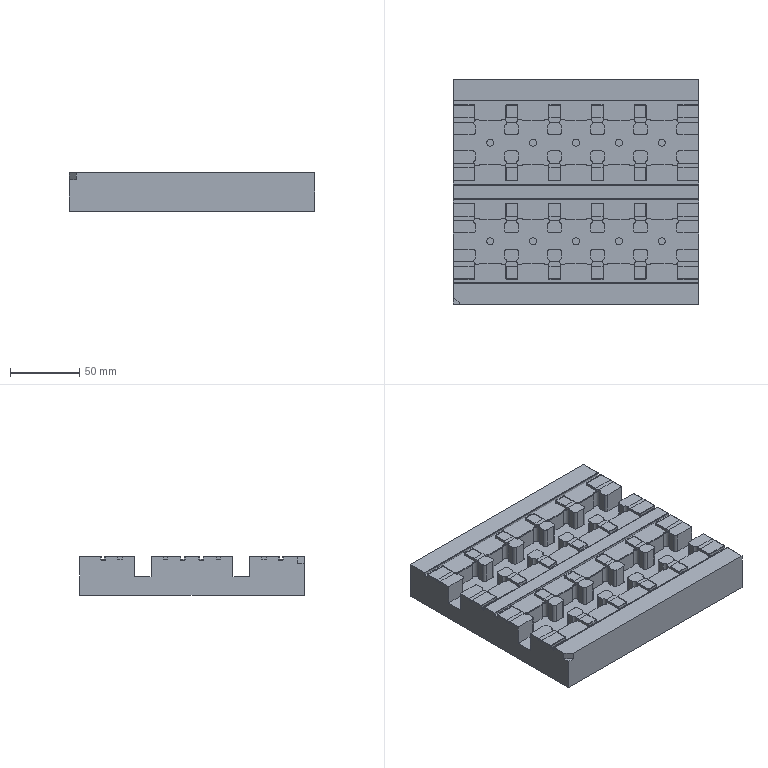NC program | NX | posted by the shop | part box 177 x 162 x 28 mm
Lines 685 to 1998 of 240480:
N4 T10 M06
(D10  D=10. R=0. H=10 ce=0.15 di=0.06)
(MAX_Z=43. MIN_Z=13.56 Time=54.07M)
T05
G00 G90 G54 X96.5 Y35.6 M03 S3000
G43 H10 Z43.
M08
Z28.551
G01 Z28.051 F2000.
X89.5
Y34.75
X74.25
G03 X67.1 Y27.6 I0.0 J-7.15
G01 Y24.98
X56.9
Y27.6
G03 X49.75 Y34.75 I-7.15 J0.0
G01 X43.25
G03 X36.1 Y27.6 I0.0 J-7.15
G01 Y24.98
X25.9
Y27.6
G03 X18.75 Y34.75 I-7.15 J0.0
G01 X12.25
G03 X5.1 Y27.6 I0.0 J-7.15
G01 Y24.98
X-5.1
Y27.6
G03 X-12.25 Y34.75 I-7.15 J0.0
G01 X-18.75
G03 X-25.9 Y27.6 I0.0 J-7.15
G01 Y24.98
X-36.1
Y27.6
G03 X-43.25 Y34.75 I-7.15 J0.0
G01 X-49.75
G03 X-56.9 Y27.6 I0.0 J-7.15
G01 Y24.98
X-67.1
Y27.6
G03 X-74.25 Y34.75 I-7.15 J0.0
G01 X-89.5
Y36.45
X-74.25
G03 X-67.1 Y43.6 I0.0 J7.15
G01 Y46.22
X-56.9
Y43.6
G03 X-55.648 Y39.558 I7.15 J0.0
G01 X-61.421 Y35.6
G03 X-62. Y34.682 I11.671 J-8.
X-62.579 Y35.6 I-12.25 J-7.082
X-62. Y36.518 I-11.671 J8.
X-61.421 Y35.6 I12.25 J7.082
G01 X-55.648 Y39.558
G03 X-49.75 Y36.45 I5.898 J4.042
G01 X-43.25
G03 X-36.1 Y43.6 I0.0 J7.15
G01 Y46.22
X-25.9
Y43.6
G03 X-24.648 Y39.558 I7.15 J0.0
G01 X-30.421 Y35.6
G03 X-31. Y34.682 I11.671 J-8.
X-31.579 Y35.6 I-12.25 J-7.082
X-31. Y36.518 I-11.671 J8.
X-30.421 Y35.6 I12.25 J7.082
G01 X-24.648 Y39.558
G03 X-18.75 Y36.45 I5.898 J4.042
G01 X-12.25
G03 X-5.1 Y43.6 I0.0 J7.15
G01 Y46.22
X5.1
Y43.6
G03 X6.352 Y39.558 I7.15 J0.0
G01 X.579 Y35.6
G03 X0.0 Y34.682 I11.671 J-8.
X-.579 Y35.6 I-12.25 J-7.082
X0.0 Y36.518 I-11.671 J8.
X.579 Y35.6 I12.25 J7.082
G01 X6.352 Y39.558
G03 X12.25 Y36.45 I5.898 J4.042
G01 X18.75
G03 X25.9 Y43.6 I0.0 J7.15
G01 Y46.22
X36.1
Y43.6
G03 X37.352 Y39.558 I7.15 J0.0
G01 X31.579 Y35.6
G03 X31. Y34.682 I11.671 J-8.
X30.421 Y35.6 I-12.25 J-7.082
X31. Y36.518 I-11.671 J8.
X31.579 Y35.6 I12.25 J7.082
G01 X37.352 Y39.558
G03 X43.25 Y36.45 I5.898 J4.042
G01 X49.75
G03 X56.9 Y43.6 I0.0 J7.15
G01 Y46.22
X67.1
Y43.6
G03 X68.352 Y39.558 I7.15 J0.0
G01 X62.579 Y35.6
G03 X62. Y34.682 I11.671 J-8.
X61.421 Y35.6 I-12.25 J-7.082
X62. Y36.518 I-11.671 J8.
X62.579 Y35.6 I12.25 J7.082
G01 X68.352 Y39.558
G03 X74.25 Y36.45 I5.898 J4.042
G01 X89.5
Y35.6
Y35.1
Z28.551
G00 Z43.
X96.65 Y35.6
Z28.353
G01 Z27.853
X89.5
Y34.75
X74.25
G03 X67.1 Y27.6 I0.0 J-7.15
G01 Y24.98
X56.9
Y27.6
G03 X49.75 Y34.75 I-7.15 J0.0
G01 X43.25
G03 X36.1 Y27.6 I0.0 J-7.15
G01 Y24.98
X25.9
Y27.6
G03 X18.75 Y34.75 I-7.15 J0.0
G01 X12.25
G03 X5.1 Y27.6 I0.0 J-7.15
G01 Y24.98
X-5.1
Y27.6
G03 X-12.25 Y34.75 I-7.15 J0.0
G01 X-18.75
G03 X-25.9 Y27.6 I0.0 J-7.15
G01 Y24.98
X-36.1
Y27.6
G03 X-43.25 Y34.75 I-7.15 J0.0
G01 X-49.75
G03 X-56.9 Y27.6 I0.0 J-7.15
G01 Y24.98
X-67.1
Y27.6
G03 X-74.25 Y34.75 I-7.15 J0.0
G01 X-89.5
Y36.45
X-74.25
G03 X-67.1 Y43.6 I0.0 J7.15
G01 Y46.22
X-56.9
Y43.6
G03 X-55.648 Y39.558 I7.15 J0.0
G01 X-61.421 Y35.6
G03 X-62. Y34.682 I11.671 J-8.
X-62.579 Y35.6 I-12.25 J-7.082
X-62. Y36.518 I-11.671 J8.
X-61.421 Y35.6 I12.25 J7.082
G01 X-55.648 Y39.558
G03 X-49.75 Y36.45 I5.898 J4.042
G01 X-43.25
G03 X-36.1 Y43.6 I0.0 J7.15
G01 Y46.22
X-25.9
Y43.6
G03 X-24.648 Y39.558 I7.15 J0.0
G01 X-30.421 Y35.6
G03 X-31. Y34.682 I11.671 J-8.
X-31.579 Y35.6 I-12.25 J-7.082
X-31. Y36.518 I-11.671 J8.
X-30.421 Y35.6 I12.25 J7.082
G01 X-24.648 Y39.558
G03 X-18.75 Y36.45 I5.898 J4.042
G01 X-12.25
G03 X-5.1 Y43.6 I0.0 J7.15
G01 Y46.22
X5.1
Y43.6
G03 X6.352 Y39.558 I7.15 J0.0
G01 X.579 Y35.6
G03 X0.0 Y34.682 I11.671 J-8.
X-.579 Y35.6 I-12.25 J-7.082
X0.0 Y36.518 I-11.671 J8.
X.579 Y35.6 I12.25 J7.082
G01 X6.352 Y39.558
G03 X12.25 Y36.45 I5.898 J4.042
G01 X18.75
G03 X25.9 Y43.6 I0.0 J7.15
G01 Y46.22
X36.1
Y43.6
G03 X37.352 Y39.558 I7.15 J0.0
G01 X31.579 Y35.6
G03 X31. Y34.682 I11.671 J-8.
X30.421 Y35.6 I-12.25 J-7.082
X31. Y36.518 I-11.671 J8.
X31.579 Y35.6 I12.25 J7.082
G01 X37.352 Y39.558
G03 X43.25 Y36.45 I5.898 J4.042
G01 X49.75
G03 X56.9 Y43.6 I0.0 J7.15
G01 Y46.22
X67.1
Y43.6
G03 X68.352 Y39.558 I7.15 J0.0
G01 X62.579 Y35.6
G03 X62. Y34.682 I11.671 J-8.
X61.421 Y35.6 I-12.25 J-7.082
X62. Y36.518 I-11.671 J8.
X62.579 Y35.6 I12.25 J7.082
G01 X68.352 Y39.558
G03 X74.25 Y36.45 I5.898 J4.042
G01 X89.5
Y35.6
Y35.1
Z28.353
G00 Z28.551
X96.65 Y35.6
Z28.154
G01 Z27.654
X89.5
Y34.75
X74.25
G03 X67.1 Y27.6 I0.0 J-7.15
G01 Y24.98
X56.9
Y27.6
G03 X49.75 Y34.75 I-7.15 J0.0
G01 X43.25
G03 X36.1 Y27.6 I0.0 J-7.15
G01 Y24.98
X25.9
Y27.6
G03 X18.75 Y34.75 I-7.15 J0.0
G01 X12.25
G03 X5.1 Y27.6 I0.0 J-7.15
G01 Y24.98
X-5.1
Y27.6
G03 X-12.25 Y34.75 I-7.15 J0.0
G01 X-18.75
G03 X-25.9 Y27.6 I0.0 J-7.15
G01 Y24.98
X-36.1
Y27.6
G03 X-43.25 Y34.75 I-7.15 J0.0
G01 X-49.75
G03 X-56.9 Y27.6 I0.0 J-7.15
G01 Y24.98
X-67.1
Y27.6
G03 X-74.25 Y34.75 I-7.15 J0.0
G01 X-89.5
Y36.45
X-74.25
G03 X-67.1 Y43.6 I0.0 J7.15
G01 Y46.22
X-56.9
Y43.6
G03 X-55.648 Y39.558 I7.15 J0.0
G01 X-61.421 Y35.6
G03 X-62. Y34.682 I11.671 J-8.
X-62.579 Y35.6 I-12.25 J-7.082
X-62. Y36.518 I-11.671 J8.
X-61.421 Y35.6 I12.25 J7.082
G01 X-55.648 Y39.558
G03 X-49.75 Y36.45 I5.898 J4.042
G01 X-43.25
G03 X-36.1 Y43.6 I0.0 J7.15
G01 Y46.22
X-25.9
Y43.6
G03 X-24.648 Y39.558 I7.15 J0.0
G01 X-30.421 Y35.6
G03 X-31. Y34.682 I11.671 J-8.
X-31.579 Y35.6 I-12.25 J-7.082
X-31. Y36.518 I-11.671 J8.
X-30.421 Y35.6 I12.25 J7.082
G01 X-24.648 Y39.558
G03 X-18.75 Y36.45 I5.898 J4.042
G01 X-12.25
G03 X-5.1 Y43.6 I0.0 J7.15
G01 Y46.22
X5.1
Y43.6
G03 X6.352 Y39.558 I7.15 J0.0
G01 X.579 Y35.6
G03 X0.0 Y34.682 I11.671 J-8.
X-.579 Y35.6 I-12.25 J-7.082
X0.0 Y36.518 I-11.671 J8.
X.579 Y35.6 I12.25 J7.082
G01 X6.352 Y39.558
G03 X12.25 Y36.45 I5.898 J4.042
G01 X18.75
G03 X25.9 Y43.6 I0.0 J7.15
G01 Y46.22
X36.1
Y43.6
G03 X37.352 Y39.558 I7.15 J0.0
G01 X31.579 Y35.6
G03 X31. Y34.682 I11.671 J-8.
X30.421 Y35.6 I-12.25 J-7.082
X31. Y36.518 I-11.671 J8.
X31.579 Y35.6 I12.25 J7.082
G01 X37.352 Y39.558
G03 X43.25 Y36.45 I5.898 J4.042
G01 X49.75
G03 X56.9 Y43.6 I0.0 J7.15
G01 Y46.22
X67.1
Y43.6
G03 X68.352 Y39.558 I7.15 J0.0
G01 X62.579 Y35.6
G03 X62. Y34.682 I11.671 J-8.
X61.421 Y35.6 I-12.25 J-7.082
X62. Y36.518 I-11.671 J8.
X62.579 Y35.6 I12.25 J7.082
G01 X68.352 Y39.558
G03 X74.25 Y36.45 I5.898 J4.042
G01 X89.5
Y35.6
Y35.1
Z28.154
G00 Z28.353
X96.65 Y35.6
Z27.956
G01 Z27.456
X89.5
Y34.75
X74.25
G03 X67.1 Y27.6 I0.0 J-7.15
G01 Y24.98
X56.9
Y27.6
G03 X49.75 Y34.75 I-7.15 J0.0
G01 X43.25
G03 X36.1 Y27.6 I0.0 J-7.15
G01 Y24.98
X25.9
Y27.6
G03 X18.75 Y34.75 I-7.15 J0.0
G01 X12.25
G03 X5.1 Y27.6 I0.0 J-7.15
G01 Y24.98
X-5.1
Y27.6
G03 X-12.25 Y34.75 I-7.15 J0.0
G01 X-18.75
G03 X-25.9 Y27.6 I0.0 J-7.15
G01 Y24.98
X-36.1
Y27.6
G03 X-43.25 Y34.75 I-7.15 J0.0
G01 X-49.75
G03 X-56.9 Y27.6 I0.0 J-7.15
G01 Y24.98
X-67.1
Y27.6
G03 X-74.25 Y34.75 I-7.15 J0.0
G01 X-89.5
Y36.45
X-74.25
G03 X-67.1 Y43.6 I0.0 J7.15
G01 Y46.22
X-56.9
Y43.6
G03 X-55.648 Y39.558 I7.15 J0.0
G01 X-61.421 Y35.6
G03 X-62. Y34.682 I11.671 J-8.
X-62.579 Y35.6 I-12.25 J-7.082
X-62. Y36.518 I-11.671 J8.
X-61.421 Y35.6 I12.25 J7.082
G01 X-55.648 Y39.558
G03 X-49.75 Y36.45 I5.898 J4.042
G01 X-43.25
G03 X-36.1 Y43.6 I0.0 J7.15
G01 Y46.22
X-25.9
Y43.6
G03 X-24.648 Y39.558 I7.15 J0.0
G01 X-30.421 Y35.6
G03 X-31. Y34.682 I11.671 J-8.
X-31.579 Y35.6 I-12.25 J-7.082
X-31. Y36.518 I-11.671 J8.
X-30.421 Y35.6 I12.25 J7.082
G01 X-24.648 Y39.558
G03 X-18.75 Y36.45 I5.898 J4.042
G01 X-12.25
G03 X-5.1 Y43.6 I0.0 J7.15
G01 Y46.22
X5.1
Y43.6
G03 X6.352 Y39.558 I7.15 J0.0
G01 X.579 Y35.6
G03 X0.0 Y34.682 I11.671 J-8.
X-.579 Y35.6 I-12.25 J-7.082
X0.0 Y36.518 I-11.671 J8.
X.579 Y35.6 I12.25 J7.082
G01 X6.352 Y39.558
G03 X12.25 Y36.45 I5.898 J4.042
G01 X18.75
G03 X25.9 Y43.6 I0.0 J7.15
G01 Y46.22
X36.1
Y43.6
G03 X37.352 Y39.558 I7.15 J0.0
G01 X31.579 Y35.6
G03 X31. Y34.682 I11.671 J-8.
X30.421 Y35.6 I-12.25 J-7.082
X31. Y36.518 I-11.671 J8.
X31.579 Y35.6 I12.25 J7.082
G01 X37.352 Y39.558
G03 X43.25 Y36.45 I5.898 J4.042
G01 X49.75
G03 X56.9 Y43.6 I0.0 J7.15
G01 Y46.22
X67.1
Y43.6
G03 X68.352 Y39.558 I7.15 J0.0
G01 X62.579 Y35.6
G03 X62. Y34.682 I11.671 J-8.
X61.421 Y35.6 I-12.25 J-7.082
X62. Y36.518 I-11.671 J8.
X62.579 Y35.6 I12.25 J7.082
G01 X68.352 Y39.558
G03 X74.25 Y36.45 I5.898 J4.042
G01 X89.5
Y35.6
Y35.1
Z27.956
G00 Z28.154
X96.65 Y35.6
Z27.757
G01 Z27.257
X89.5
Y34.75
X74.25
G03 X67.1 Y27.6 I0.0 J-7.15
G01 Y24.98
X56.9
Y27.6
G03 X49.75 Y34.75 I-7.15 J0.0
G01 X43.25
G03 X36.1 Y27.6 I0.0 J-7.15
G01 Y24.98
X25.9
Y27.6
G03 X18.75 Y34.75 I-7.15 J0.0
G01 X12.25
G03 X5.1 Y27.6 I0.0 J-7.15
G01 Y24.98
X-5.1
Y27.6
G03 X-12.25 Y34.75 I-7.15 J0.0
G01 X-18.75
G03 X-25.9 Y27.6 I0.0 J-7.15
G01 Y24.98
X-36.1
Y27.6
G03 X-43.25 Y34.75 I-7.15 J0.0
G01 X-49.75
G03 X-56.9 Y27.6 I0.0 J-7.15
G01 Y24.98
X-67.1
Y27.6
G03 X-74.25 Y34.75 I-7.15 J0.0
G01 X-89.5
Y36.45
X-74.25
G03 X-67.1 Y43.6 I0.0 J7.15
G01 Y46.22
X-56.9
Y43.6
G03 X-55.648 Y39.558 I7.15 J0.0
G01 X-61.421 Y35.6
G03 X-62. Y34.682 I11.671 J-8.
X-62.579 Y35.6 I-12.25 J-7.082
X-62. Y36.518 I-11.671 J8.
X-61.421 Y35.6 I12.25 J7.082
G01 X-55.648 Y39.558
G03 X-49.75 Y36.45 I5.898 J4.042
G01 X-43.25
G03 X-36.1 Y43.6 I0.0 J7.15
G01 Y46.22
X-25.9
Y43.6
G03 X-24.648 Y39.558 I7.15 J0.0
G01 X-30.421 Y35.6
G03 X-31. Y34.682 I11.671 J-8.
X-31.579 Y35.6 I-12.25 J-7.082
X-31. Y36.518 I-11.671 J8.
X-30.421 Y35.6 I12.25 J7.082
G01 X-24.648 Y39.558
G03 X-18.75 Y36.45 I5.898 J4.042
G01 X-12.25
G03 X-5.1 Y43.6 I0.0 J7.15
G01 Y46.22
X5.1
Y43.6
G03 X6.352 Y39.558 I7.15 J0.0
G01 X.579 Y35.6
G03 X0.0 Y34.682 I11.671 J-8.
X-.579 Y35.6 I-12.25 J-7.082
X0.0 Y36.518 I-11.671 J8.
X.579 Y35.6 I12.25 J7.082
G01 X6.352 Y39.558
G03 X12.25 Y36.45 I5.898 J4.042
G01 X18.75
G03 X25.9 Y43.6 I0.0 J7.15
G01 Y46.22
X36.1
Y43.6
G03 X37.352 Y39.558 I7.15 J0.0
G01 X31.579 Y35.6
G03 X31. Y34.682 I11.671 J-8.
X30.421 Y35.6 I-12.25 J-7.082
X31. Y36.518 I-11.671 J8.
X31.579 Y35.6 I12.25 J7.082
G01 X37.352 Y39.558
G03 X43.25 Y36.45 I5.898 J4.042
G01 X49.75
G03 X56.9 Y43.6 I0.0 J7.15
G01 Y46.22
X67.1
Y43.6
G03 X68.352 Y39.558 I7.15 J0.0
G01 X62.579 Y35.6
G03 X62. Y34.682 I11.671 J-8.
X61.421 Y35.6 I-12.25 J-7.082
X62. Y36.518 I-11.671 J8.
X62.579 Y35.6 I12.25 J7.082
G01 X68.352 Y39.558
G03 X74.25 Y36.45 I5.898 J4.042
G01 X89.5
Y35.6
Y35.1
Z27.757
G00 Z27.956
X96.65 Y35.6
Z27.559
G01 Z27.059
X89.5
Y34.75
X74.25
G03 X67.1 Y27.6 I0.0 J-7.15
G01 Y24.98
X56.9
Y27.6
G03 X49.75 Y34.75 I-7.15 J0.0
G01 X43.25
G03 X36.1 Y27.6 I0.0 J-7.15
G01 Y24.98
X25.9
Y27.6
G03 X18.75 Y34.75 I-7.15 J0.0
G01 X12.25
G03 X5.1 Y27.6 I0.0 J-7.15
G01 Y24.98
X-5.1
Y27.6
G03 X-12.25 Y34.75 I-7.15 J0.0
G01 X-18.75
G03 X-25.9 Y27.6 I0.0 J-7.15
G01 Y24.98
X-36.1
Y27.6
G03 X-43.25 Y34.75 I-7.15 J0.0
G01 X-49.75
G03 X-56.9 Y27.6 I0.0 J-7.15
G01 Y24.98
X-67.1
Y27.6
G03 X-74.25 Y34.75 I-7.15 J0.0
G01 X-89.5
Y36.45
X-74.25
G03 X-67.1 Y43.6 I0.0 J7.15
G01 Y46.22
X-56.9
Y43.6
G03 X-55.648 Y39.558 I7.15 J0.0
G01 X-61.421 Y35.6
G03 X-62. Y34.682 I11.671 J-8.
X-62.579 Y35.6 I-12.25 J-7.082
X-62. Y36.518 I-11.671 J8.
X-61.421 Y35.6 I12.25 J7.082
G01 X-55.648 Y39.558
G03 X-49.75 Y36.45 I5.898 J4.042
G01 X-43.25
G03 X-36.1 Y43.6 I0.0 J7.15
G01 Y46.22
X-25.9
Y43.6
G03 X-24.648 Y39.558 I7.15 J0.0
G01 X-30.421 Y35.6
G03 X-31. Y34.682 I11.671 J-8.
X-31.579 Y35.6 I-12.25 J-7.082
X-31. Y36.518 I-11.671 J8.
X-30.421 Y35.6 I12.25 J7.082
G01 X-24.648 Y39.558
G03 X-18.75 Y36.45 I5.898 J4.042
G01 X-12.25
G03 X-5.1 Y43.6 I0.0 J7.15
G01 Y46.22
X5.1
Y43.6
G03 X6.352 Y39.558 I7.15 J0.0
G01 X.579 Y35.6
G03 X0.0 Y34.682 I11.671 J-8.
X-.579 Y35.6 I-12.25 J-7.082
X0.0 Y36.518 I-11.671 J8.
X.579 Y35.6 I12.25 J7.082
G01 X6.352 Y39.558
G03 X12.25 Y36.45 I5.898 J4.042
G01 X18.75
G03 X25.9 Y43.6 I0.0 J7.15
G01 Y46.22
X36.1
Y43.6
G03 X37.352 Y39.558 I7.15 J0.0
G01 X31.579 Y35.6
G03 X31. Y34.682 I11.671 J-8.
X30.421 Y35.6 I-12.25 J-7.082
X31. Y36.518 I-11.671 J8.
X31.579 Y35.6 I12.25 J7.082
G01 X37.352 Y39.558
G03 X43.25 Y36.45 I5.898 J4.042
G01 X49.75
G03 X56.9 Y43.6 I0.0 J7.15
G01 Y46.22
X67.1
Y43.6
G03 X68.352 Y39.558 I7.15 J0.0
G01 X62.579 Y35.6
G03 X62. Y34.682 I11.671 J-8.
X61.421 Y35.6 I-12.25 J-7.082
X62. Y36.518 I-11.671 J8.
X62.579 Y35.6 I12.25 J7.082
G01 X68.352 Y39.558
G03 X74.25 Y36.45 I5.898 J4.042
G01 X89.5
Y35.6
Y35.1
Z27.559
G00 Z27.757
X96.65 Y35.6
Z27.36
G01 Z26.86
X89.5
Y34.75
X74.25
G03 X67.1 Y27.6 I0.0 J-7.15
G01 Y24.98
X56.9
Y27.6
G03 X49.75 Y34.75 I-7.15 J0.0
G01 X43.25
G03 X36.1 Y27.6 I0.0 J-7.15
G01 Y24.98
X25.9
Y27.6
G03 X18.75 Y34.75 I-7.15 J0.0
G01 X12.25
G03 X5.1 Y27.6 I0.0 J-7.15
G01 Y24.98
X-5.1
Y27.6
G03 X-12.25 Y34.75 I-7.15 J0.0
G01 X-18.75
G03 X-25.9 Y27.6 I0.0 J-7.15
G01 Y24.98
X-36.1
Y27.6
G03 X-43.25 Y34.75 I-7.15 J0.0
G01 X-49.75
G03 X-56.9 Y27.6 I0.0 J-7.15
G01 Y24.98
X-67.1
Y27.6
G03 X-74.25 Y34.75 I-7.15 J0.0
G01 X-89.5
Y36.45
X-74.25
G03 X-67.1 Y43.6 I0.0 J7.15
G01 Y46.22
X-56.9
Y43.6
G03 X-55.648 Y39.558 I7.15 J0.0
G01 X-61.421 Y35.6
G03 X-62. Y34.682 I11.671 J-8.
X-62.579 Y35.6 I-12.25 J-7.082
X-62. Y36.518 I-11.671 J8.
X-61.421 Y35.6 I12.25 J7.082
G01 X-55.648 Y39.558
G03 X-49.75 Y36.45 I5.898 J4.042
G01 X-43.25
G03 X-36.1 Y43.6 I0.0 J7.15
G01 Y46.22
X-25.9
Y43.6
G03 X-24.648 Y39.558 I7.15 J0.0
G01 X-30.421 Y35.6
G03 X-31. Y34.682 I11.671 J-8.
X-31.579 Y35.6 I-12.25 J-7.082
X-31. Y36.518 I-11.671 J8.
X-30.421 Y35.6 I12.25 J7.082
G01 X-24.648 Y39.558
G03 X-18.75 Y36.45 I5.898 J4.042
G01 X-12.25
G03 X-5.1 Y43.6 I0.0 J7.15
G01 Y46.22
X5.1
Y43.6
G03 X6.352 Y39.558 I7.15 J0.0
G01 X.579 Y35.6
G03 X0.0 Y34.682 I11.671 J-8.
X-.579 Y35.6 I-12.25 J-7.082
X0.0 Y36.518 I-11.671 J8.
X.579 Y35.6 I12.25 J7.082
G01 X6.352 Y39.558
G03 X12.25 Y36.45 I5.898 J4.042
G01 X18.75
G03 X25.9 Y43.6 I0.0 J7.15
G01 Y46.22
X36.1
Y43.6
G03 X37.352 Y39.558 I7.15 J0.0
G01 X31.579 Y35.6
G03 X31. Y34.682 I11.671 J-8.
X30.421 Y35.6 I-12.25 J-7.082
X31. Y36.518 I-11.671 J8.
X31.579 Y35.6 I12.25 J7.082
G01 X37.352 Y39.558
G03 X43.25 Y36.45 I5.898 J4.042
G01 X49.75
G03 X56.9 Y43.6 I0.0 J7.15
G01 Y46.22
X67.1
Y43.6
G03 X68.352 Y39.558 I7.15 J0.0
G01 X62.579 Y35.6
G03 X62. Y34.682 I11.671 J-8.
X61.421 Y35.6 I-12.25 J-7.082
X62. Y36.518 I-11.671 J8.
X62.579 Y35.6 I12.25 J7.082
G01 X68.352 Y39.558
G03 X74.25 Y36.45 I5.898 J4.042
G01 X89.5
Y35.6
Y35.1
Z27.36
G00 Z27.559
X96.65 Y35.6
Z27.162
G01 Z26.662
X89.5
Y34.75
X74.25
G03 X67.1 Y27.6 I0.0 J-7.15
G01 Y24.98
X56.9
Y27.6
G03 X49.75 Y34.75 I-7.15 J0.0
G01 X43.25
G03 X36.1 Y27.6 I0.0 J-7.15
G01 Y24.98
X25.9
Y27.6
G03 X18.75 Y34.75 I-7.15 J0.0
G01 X12.25
G03 X5.1 Y27.6 I0.0 J-7.15
G01 Y24.98
X-5.1
Y27.6
G03 X-12.25 Y34.75 I-7.15 J0.0
G01 X-18.75
G03 X-25.9 Y27.6 I0.0 J-7.15
G01 Y24.98
X-36.1
Y27.6
G03 X-43.25 Y34.75 I-7.15 J0.0
G01 X-49.75
G03 X-56.9 Y27.6 I0.0 J-7.15
G01 Y24.98
X-67.1
Y27.6
G03 X-74.25 Y34.75 I-7.15 J0.0
G01 X-89.5
Y36.45
X-74.25
G03 X-67.1 Y43.6 I0.0 J7.15
G01 Y46.22
X-56.9
Y43.6
G03 X-55.648 Y39.558 I7.15 J0.0
G01 X-61.421 Y35.6
G03 X-62. Y34.682 I11.671 J-8.
X-62.579 Y35.6 I-12.25 J-7.082
X-62. Y36.518 I-11.671 J8.
X-61.421 Y35.6 I12.25 J7.082
G01 X-55.648 Y39.558
G03 X-49.75 Y36.45 I5.898 J4.042
G01 X-43.25
G03 X-36.1 Y43.6 I0.0 J7.15
G01 Y46.22
X-25.9
Y43.6
G03 X-24.648 Y39.558 I7.15 J0.0
G01 X-30.421 Y35.6
G03 X-31. Y34.682 I11.671 J-8.
X-31.579 Y35.6 I-12.25 J-7.082
X-31. Y36.518 I-11.671 J8.
X-30.421 Y35.6 I12.25 J7.082
G01 X-24.648 Y39.558
G03 X-18.75 Y36.45 I5.898 J4.042
G01 X-12.25
G03 X-5.1 Y43.6 I0.0 J7.15
G01 Y46.22
X5.1
Y43.6
G03 X6.352 Y39.558 I7.15 J0.0
G01 X.579 Y35.6
G03 X0.0 Y34.682 I11.671 J-8.
X-.579 Y35.6 I-12.25 J-7.082
X0.0 Y36.518 I-11.671 J8.
X.579 Y35.6 I12.25 J7.082
G01 X6.352 Y39.558
G03 X12.25 Y36.45 I5.898 J4.042
G01 X18.75
G03 X25.9 Y43.6 I0.0 J7.15
G01 Y46.22
X36.1
Y43.6
G03 X37.352 Y39.558 I7.15 J0.0
G01 X31.579 Y35.6
G03 X31. Y34.682 I11.671 J-8.
X30.421 Y35.6 I-12.25 J-7.082
X31. Y36.518 I-11.671 J8.
X31.579 Y35.6 I12.25 J7.082
G01 X37.352 Y39.558
G03 X43.25 Y36.45 I5.898 J4.042
G01 X49.75
G03 X56.9 Y43.6 I0.0 J7.15
G01 Y46.22
X67.1
Y43.6
G03 X68.352 Y39.558 I7.15 J0.0
G01 X62.579 Y35.6
G03 X62. Y34.682 I11.671 J-8.
X61.421 Y35.6 I-12.25 J-7.082
X62. Y36.518 I-11.671 J8.
X62.579 Y35.6 I12.25 J7.082
G01 X68.352 Y39.558
G03 X74.25 Y36.45 I5.898 J4.042
G01 X89.5
Y35.6
Y35.1
Z27.162
G00 Z27.36
X96.65 Y35.6
Z26.963
G01 Z26.463
X89.5
Y34.75
X74.25
G03 X67.1 Y27.6 I0.0 J-7.15
G01 Y24.98
X56.9
Y27.6
G03 X49.75 Y34.75 I-7.15 J0.0
G01 X43.25
G03 X36.1 Y27.6 I0.0 J-7.15
G01 Y24.98
X25.9
Y27.6
G03 X18.75 Y34.75 I-7.15 J0.0
G01 X12.25
G03 X5.1 Y27.6 I0.0 J-7.15
G01 Y24.98
X-5.1
Y27.6
G03 X-12.25 Y34.75 I-7.15 J0.0
G01 X-18.75
G03 X-25.9 Y27.6 I0.0 J-7.15
G01 Y24.98
X-36.1
Y27.6
G03 X-43.25 Y34.75 I-7.15 J0.0
G01 X-49.75
G03 X-56.9 Y27.6 I0.0 J-7.15
G01 Y24.98
X-67.1
Y27.6
G03 X-74.25 Y34.75 I-7.15 J0.0
G01 X-89.5
Y36.45
X-74.25
G03 X-67.1 Y43.6 I0.0 J7.15
G01 Y46.22
X-56.9
Y43.6
G03 X-55.648 Y39.558 I7.15 J0.0
G01 X-61.421 Y35.6
G03 X-62. Y34.682 I11.671 J-8.
X-62.579 Y35.6 I-12.25 J-7.082
X-62. Y36.518 I-11.671 J8.
X-61.421 Y35.6 I12.25 J7.082
G01 X-55.648 Y39.558
G03 X-49.75 Y36.45 I5.898 J4.042
G01 X-43.25
G03 X-36.1 Y43.6 I0.0 J7.15
G01 Y46.22
X-25.9
Y43.6
G03 X-24.648 Y39.558 I7.15 J0.0
G01 X-30.421 Y35.6
G03 X-31. Y34.682 I11.671 J-8.
X-31.579 Y35.6 I-12.25 J-7.082
X-31. Y36.518 I-11.671 J8.
X-30.421 Y35.6 I12.25 J7.082
G01 X-24.648 Y39.558
G03 X-18.75 Y36.45 I5.898 J4.042
G01 X-12.25
G03 X-5.1 Y43.6 I0.0 J7.15
G01 Y46.22
X5.1
Y43.6
G03 X6.352 Y39.558 I7.15 J0.0
G01 X.579 Y35.6
G03 X0.0 Y34.682 I11.671 J-8.
X-.579 Y35.6 I-12.25 J-7.082
X0.0 Y36.518 I-11.671 J8.
X.579 Y35.6 I12.25 J7.082
G01 X6.352 Y39.558
G03 X12.25 Y36.45 I5.898 J4.042
G01 X18.75
G03 X25.9 Y43.6 I0.0 J7.15
G01 Y46.22
X36.1
Y43.6
G03 X37.352 Y39.558 I7.15 J0.0
G01 X31.579 Y35.6
G03 X31. Y34.682 I11.671 J-8.
X30.421 Y35.6 I-12.25 J-7.082
X31. Y36.518 I-11.671 J8.
X31.579 Y35.6 I12.25 J7.082
G01 X37.352 Y39.558
G03 X43.25 Y36.45 I5.898 J4.042
G01 X49.75
G03 X56.9 Y43.6 I0.0 J7.15
G01 Y46.22
X67.1
Y43.6
G03 X68.352 Y39.558 I7.15 J0.0
G01 X62.579 Y35.6
G03 X62. Y34.682 I11.671 J-8.
X61.421 Y35.6 I-12.25 J-7.082
X62. Y36.518 I-11.671 J8.
X62.579 Y35.6 I12.25 J7.082
G01 X68.352 Y39.558
G03 X74.25 Y36.45 I5.898 J4.042
G01 X89.5
Y35.6
Y35.1
Z26.963
G00 Z27.162
X96.65 Y35.6
Z26.765
G01 Z26.265
X89.5
Y34.75
X74.25
G03 X67.1 Y27.6 I0.0 J-7.15
G01 Y24.98
X56.9
Y27.6
G03 X49.75 Y34.75 I-7.15 J0.0
G01 X43.25
G03 X36.1 Y27.6 I0.0 J-7.15
G01 Y24.98
X25.9
Y27.6
G03 X18.75 Y34.75 I-7.15 J0.0
G01 X12.25
G03 X5.1 Y27.6 I0.0 J-7.15
G01 Y24.98
X-5.1
Y27.6
G03 X-12.25 Y34.75 I-7.15 J0.0
G01 X-18.75
G03 X-25.9 Y27.6 I0.0 J-7.15
G01 Y24.98
X-36.1
Y27.6
G03 X-43.25 Y34.75 I-7.15 J0.0
G01 X-49.75
G03 X-56.9 Y27.6 I0.0 J-7.15
G01 Y24.98
X-67.1
Y27.6
G03 X-74.25 Y34.75 I-7.15 J0.0
G01 X-89.5
Y36.45
X-74.25
G03 X-67.1 Y43.6 I0.0 J7.15
G01 Y46.22
X-56.9
Y43.6
G03 X-55.648 Y39.558 I7.15 J0.0
G01 X-61.421 Y35.6
G03 X-62. Y34.682 I11.671 J-8.
X-62.579 Y35.6 I-12.25 J-7.082
X-62. Y36.518 I-11.671 J8.
X-61.421 Y35.6 I12.25 J7.082
G01 X-55.648 Y39.558
G03 X-49.75 Y36.45 I5.898 J4.042
G01 X-43.25
G03 X-36.1 Y43.6 I0.0 J7.15
G01 Y46.22
X-25.9
Y43.6
G03 X-24.648 Y39.558 I7.15 J0.0
G01 X-30.421 Y35.6
G03 X-31. Y34.682 I11.671 J-8.
X-31.579 Y35.6 I-12.25 J-7.082
X-31. Y36.518 I-11.671 J8.
X-30.421 Y35.6 I12.25 J7.082
G01 X-24.648 Y39.558
G03 X-18.75 Y36.45 I5.898 J4.042
G01 X-12.25
G03 X-5.1 Y43.6 I0.0 J7.15
G01 Y46.22
X5.1
Y43.6
G03 X6.352 Y39.558 I7.15 J0.0
G01 X.579 Y35.6
G03 X0.0 Y34.682 I11.671 J-8.
X-.579 Y35.6 I-12.25 J-7.082
X0.0 Y36.518 I-11.671 J8.
X.579 Y35.6 I12.25 J7.082
G01 X6.352 Y39.558
G03 X12.25 Y36.45 I5.898 J4.042
G01 X18.75
G03 X25.9 Y43.6 I0.0 J7.15
G01 Y46.22
X36.1
Y43.6
G03 X37.352 Y39.558 I7.15 J0.0
G01 X31.579 Y35.6
G03 X31. Y34.682 I11.671 J-8.
X30.421 Y35.6 I-12.25 J-7.082
X31. Y36.518 I-11.671 J8.
X31.579 Y35.6 I12.25 J7.082
G01 X37.352 Y39.558
G03 X43.25 Y36.45 I5.898 J4.042
G01 X49.75
G03 X56.9 Y43.6 I0.0 J7.15
G01 Y46.22
X67.1
Y43.6
G03 X68.352 Y39.558 I7.15 J0.0
G01 X62.579 Y35.6
G03 X62. Y34.682 I11.671 J-8.
X61.421 Y35.6 I-12.25 J-7.082
X62. Y36.518 I-11.671 J8.
X62.579 Y35.6 I12.25 J7.082
G01 X68.352 Y39.558
G03 X74.25 Y36.45 I5.898 J4.042
G01 X89.5
Y35.6
Y35.1
Z26.765
G00 Z26.963
X96.65 Y35.6
Z26.566
G01 Z26.066
X89.5
Y34.75
X74.25
G03 X67.1 Y27.6 I0.0 J-7.15
G01 Y24.98
X56.9
Y27.6
G03 X49.75 Y34.75 I-7.15 J0.0
G01 X43.25
G03 X36.1 Y27.6 I0.0 J-7.15
G01 Y24.98
X25.9
Y27.6
G03 X18.75 Y34.75 I-7.15 J0.0
G01 X12.25
G03 X5.1 Y27.6 I0.0 J-7.15
G01 Y24.98
X-5.1
Y27.6
G03 X-12.25 Y34.75 I-7.15 J0.0
G01 X-18.75
G03 X-25.9 Y27.6 I0.0 J-7.15
G01 Y24.98
X-36.1
Y27.6
G03 X-43.25 Y34.75 I-7.15 J0.0
G01 X-49.75
G03 X-56.9 Y27.6 I0.0 J-7.15
G01 Y24.98
X-67.1
Y27.6
G03 X-74.25 Y34.75 I-7.15 J0.0
G01 X-89.5
Y36.45
X-74.25
G03 X-67.1 Y43.6 I0.0 J7.15
G01 Y46.22
X-56.9
Y43.6
G03 X-55.648 Y39.558 I7.15 J0.0
G01 X-61.421 Y35.6
G03 X-62. Y34.682 I11.671 J-8.
X-62.579 Y35.6 I-12.25 J-7.082
X-62. Y36.518 I-11.671 J8.
X-61.421 Y35.6 I12.25 J7.082
G01 X-55.648 Y39.558
G03 X-49.75 Y36.45 I5.898 J4.042
G01 X-43.25
G03 X-36.1 Y43.6 I0.0 J7.15
G01 Y46.22
X-25.9
Y43.6
G03 X-24.648 Y39.558 I7.15 J0.0
G01 X-30.421 Y35.6
G03 X-31. Y34.682 I11.671 J-8.
X-31.579 Y35.6 I-12.25 J-7.082
X-31. Y36.518 I-11.671 J8.
X-30.421 Y35.6 I12.25 J7.082
G01 X-24.648 Y39.558
G03 X-18.75 Y36.45 I5.898 J4.042
G01 X-12.25
G03 X-5.1 Y43.6 I0.0 J7.15
G01 Y46.22
X5.1
Y43.6
G03 X6.352 Y39.558 I7.15 J0.0
G01 X.579 Y35.6
G03 X0.0 Y34.682 I11.671 J-8.
X-.579 Y35.6 I-12.25 J-7.082
X0.0 Y36.518 I-11.671 J8.
X.579 Y35.6 I12.25 J7.082
G01 X6.352 Y39.558
G03 X12.25 Y36.45 I5.898 J4.042
G01 X18.75
G03 X25.9 Y43.6 I0.0 J7.15
G01 Y46.22
X36.1
Y43.6
G03 X37.352 Y39.558 I7.15 J0.0
G01 X31.579 Y35.6
G03 X31. Y34.682 I11.671 J-8.
X30.421 Y35.6 I-12.25 J-7.082
X31. Y36.518 I-11.671 J8.
X31.579 Y35.6 I12.25 J7.082
G01 X37.352 Y39.558
G03 X43.25 Y36.45 I5.898 J4.042
G01 X49.75
G03 X56.9 Y43.6 I0.0 J7.15
G01 Y46.22
X67.1
Y43.6
G03 X68.352 Y39.558 I7.15 J0.0
G01 X62.579 Y35.6
G03 X62. Y34.682 I11.671 J-8.
X61.421 Y35.6 I-12.25 J-7.082
X62. Y36.518 I-11.671 J8.
X62.579 Y35.6 I12.25 J7.082
G01 X68.352 Y39.558
G03 X74.25 Y36.45 I5.898 J4.042
G01 X89.5
Y35.6
Y35.1
Z26.566
G00 Z26.765
X96.65 Y35.6
Z26.368
G01 Z25.868
X89.5
Y34.75
X74.25
G03 X67.1 Y27.6 I0.0 J-7.15
G01 Y24.98
X56.9
Y27.6
G03 X49.75 Y34.75 I-7.15 J0.0
G01 X43.25
G03 X36.1 Y27.6 I0.0 J-7.15
G01 Y24.98
X25.9
Y27.6
G03 X18.75 Y34.75 I-7.15 J0.0
G01 X12.25
G03 X5.1 Y27.6 I0.0 J-7.15
G01 Y24.98
X-5.1
Y27.6
G03 X-12.25 Y34.75 I-7.15 J0.0
G01 X-18.75
G03 X-25.9 Y27.6 I0.0 J-7.15
G01 Y24.98
X-36.1
Y27.6
G03 X-43.25 Y34.75 I-7.15 J0.0
G01 X-49.75
G03 X-56.9 Y27.6 I0.0 J-7.15
G01 Y24.98
X-67.1
Y27.6
G03 X-74.25 Y34.75 I-7.15 J0.0
G01 X-89.5
Y36.45
X-74.25
G03 X-67.1 Y43.6 I0.0 J7.15
G01 Y46.22
X-56.9
Y43.6
G03 X-55.648 Y39.558 I7.15 J0.0
G01 X-61.421 Y35.6
G03 X-62. Y34.682 I11.671 J-8.
X-62.579 Y35.6 I-12.25 J-7.082
X-62. Y36.518 I-11.671 J8.
X-61.421 Y35.6 I12.25 J7.082
G01 X-55.648 Y39.558
G03 X-49.75 Y36.45 I5.898 J4.042
G01 X-43.25
G03 X-36.1 Y43.6 I0.0 J7.15
G01 Y46.22
X-25.9
Y43.6
G03 X-24.648 Y39.558 I7.15 J0.0
G01 X-30.421 Y35.6
G03 X-31. Y34.682 I11.671 J-8.
X-31.579 Y35.6 I-12.25 J-7.082
X-31. Y36.518 I-11.671 J8.
X-30.421 Y35.6 I12.25 J7.082
G01 X-24.648 Y39.558
G03 X-18.75 Y36.45 I5.898 J4.042
G01 X-12.25
G03 X-5.1 Y43.6 I0.0 J7.15
G01 Y46.22
X5.1
Y43.6
G03 X6.352 Y39.558 I7.15 J0.0
G01 X.579 Y35.6
G03 X0.0 Y34.682 I11.671 J-8.
X-.579 Y35.6 I-12.25 J-7.082
X0.0 Y36.518 I-11.671 J8.
X.579 Y35.6 I12.25 J7.082
G01 X6.352 Y39.558
G03 X12.25 Y36.45 I5.898 J4.042
G01 X18.75
G03 X25.9 Y43.6 I0.0 J7.15
G01 Y46.22
X36.1
Y43.6
G03 X37.352 Y39.558 I7.15 J0.0
G01 X31.579 Y35.6
G03 X31. Y34.682 I11.671 J-8.
X30.421 Y35.6 I-12.25 J-7.082
X31. Y36.518 I-11.671 J8.
X31.579 Y35.6 I12.25 J7.082
G01 X37.352 Y39.558
G03 X43.25 Y36.45 I5.898 J4.042
G01 X49.75
G03 X56.9 Y43.6 I0.0 J7.15
G01 Y46.22
X67.1
Y43.6
G03 X68.352 Y39.558 I7.15 J0.0
G01 X62.579 Y35.6
G03 X62. Y34.682 I11.671 J-8.
X61.421 Y35.6 I-12.25 J-7.082
X62. Y36.518 I-11.671 J8.
X62.579 Y35.6 I12.25 J7.082
G01 X68.352 Y39.558
G03 X74.25 Y36.45 I5.898 J4.042
G01 X89.5
Y35.6
Y35.1
Z26.368
G00 Z26.566
X96.65 Y35.6
Z26.169
G01 Z25.669
X89.5
Y34.75
X74.25
G03 X67.1 Y27.6 I0.0 J-7.15
G01 Y24.98
X56.9
Y27.6
G03 X49.75 Y34.75 I-7.15 J0.0
G01 X43.25
G03 X36.1 Y27.6 I0.0 J-7.15
G01 Y24.98
X25.9
Y27.6
G03 X18.75 Y34.75 I-7.15 J0.0
G01 X12.25
G03 X5.1 Y27.6 I0.0 J-7.15
G01 Y24.98
X-5.1
Y27.6
G03 X-12.25 Y34.75 I-7.15 J0.0
G01 X-18.75